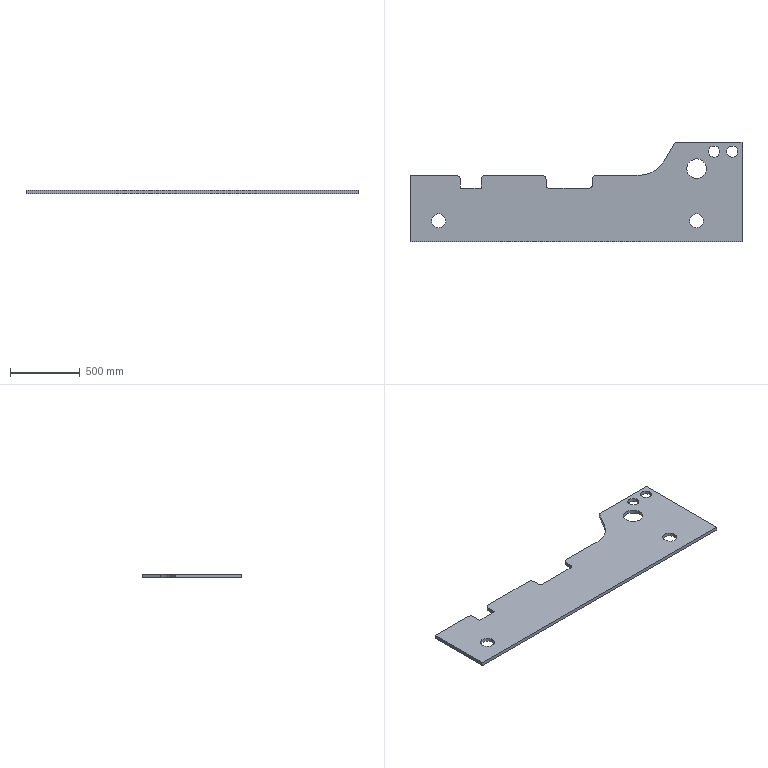Part | SolidWorks | features Extrusion 1 | 1 solid | 33 faces | box 2375 x 714.5 x 25 mm | volume 29470631 mm3 | cylinder 17 | plane 16 | commonest cylinder face diameters 60 x4 80 x4 100 x4 40 x2 140 x2 418 x1
STEP:
#1=CARTESIAN_POINT('',(155.,151.5,25.));
#2=VERTEX_POINT('',#1);
#3=CARTESIAN_POINT('',(255.,151.5,25.));
#4=VERTEX_POINT('',#3);
#5=CARTESIAN_POINT('',(205.,151.5,25.));
#6=DIRECTION('',(0.,0.,1.));
#7=DIRECTION('',(1.,0.,0.));
#8=AXIS2_PLACEMENT_3D('',#5,#6,#7);
#9=CIRCLE('',#8,50.);
#10=EDGE_CURVE('',#2,#4,#9,.T.);
#11=ORIENTED_EDGE('',*,*,#10,.T.);
#12=CARTESIAN_POINT('',(255.,151.5,0.));
#13=VERTEX_POINT('',#12);
#14=CARTESIAN_POINT('',(255.,151.5,25.));
#15=DIRECTION('',(0.,0.,-1.));
#16=VECTOR('',#15,1000.);
#17=LINE('',#14,#16);
#18=EDGE_CURVE('',#4,#13,#17,.T.);
#19=ORIENTED_EDGE('',*,*,#18,.T.);
#20=CARTESIAN_POINT('',(155.,151.5,0.));
#21=VERTEX_POINT('',#20);
#22=CARTESIAN_POINT('',(205.,151.5,0.));
#23=DIRECTION('',(0.,0.,1.));
#24=DIRECTION('',(1.,0.,0.));
#25=AXIS2_PLACEMENT_3D('',#22,#23,#24);
#26=CIRCLE('',#25,50.);
#27=EDGE_CURVE('',#21,#13,#26,.T.);
#28=ORIENTED_EDGE('',*,*,#27,.F.);
#29=CARTESIAN_POINT('',(155.,151.5,25.));
#30=DIRECTION('',(0.,0.,-1.));
#31=VECTOR('',#30,1000.);
#32=LINE('',#29,#31);
#33=EDGE_CURVE('',#2,#21,#32,.T.);
#34=ORIENTED_EDGE('',*,*,#33,.F.);
#35=EDGE_LOOP('',(#11,#19,#28,#34));
#36=FACE_OUTER_BOUND('',#35,.T.);
#37=CARTESIAN_POINT('',(205.,151.5,25.));
#38=DIRECTION('',(0.,0.,-1.));
#39=DIRECTION('',(-1.,0.,0.));
#40=AXIS2_PLACEMENT_3D('',#37,#38,#39);
#41=CYLINDRICAL_SURFACE('',#40,50.);
#42=ADVANCED_FACE('',(#36),#41,.F.);
#43=CARTESIAN_POINT('',(2135.,646.5,25.));
#44=VERTEX_POINT('',#43);
#45=CARTESIAN_POINT('',(2215.,646.5,25.));
#46=VERTEX_POINT('',#45);
#47=CARTESIAN_POINT('',(2175.,646.5,25.));
#48=DIRECTION('',(0.,0.,1.));
#49=DIRECTION('',(1.,0.,0.));
#50=AXIS2_PLACEMENT_3D('',#47,#48,#49);
#51=CIRCLE('',#50,40.);
#52=EDGE_CURVE('',#44,#46,#51,.T.);
#53=ORIENTED_EDGE('',*,*,#52,.T.);
#54=CARTESIAN_POINT('',(2215.,646.5,0.));
#55=VERTEX_POINT('',#54);
#56=CARTESIAN_POINT('',(2215.,646.5,25.));
#57=DIRECTION('',(0.,0.,-1.));
#58=VECTOR('',#57,1000.);
#59=LINE('',#56,#58);
#60=EDGE_CURVE('',#46,#55,#59,.T.);
#61=ORIENTED_EDGE('',*,*,#60,.T.);
#62=CARTESIAN_POINT('',(2135.,646.5,0.));
#63=VERTEX_POINT('',#62);
#64=CARTESIAN_POINT('',(2175.,646.5,0.));
#65=DIRECTION('',(0.,0.,1.));
#66=DIRECTION('',(1.,0.,0.));
#67=AXIS2_PLACEMENT_3D('',#64,#65,#66);
#68=CIRCLE('',#67,40.);
#69=EDGE_CURVE('',#63,#55,#68,.T.);
#70=ORIENTED_EDGE('',*,*,#69,.F.);
#71=CARTESIAN_POINT('',(2135.,646.5,25.));
#72=DIRECTION('',(0.,0.,-1.));
#73=VECTOR('',#72,1000.);
#74=LINE('',#71,#73);
#75=EDGE_CURVE('',#44,#63,#74,.T.);
#76=ORIENTED_EDGE('',*,*,#75,.F.);
#77=EDGE_LOOP('',(#53,#61,#70,#76));
#78=FACE_OUTER_BOUND('',#77,.T.);
#79=CARTESIAN_POINT('',(2175.,646.5,25.));
#80=DIRECTION('',(0.,0.,-1.));
#81=DIRECTION('',(-1.,0.,0.));
#82=AXIS2_PLACEMENT_3D('',#79,#80,#81);
#83=CYLINDRICAL_SURFACE('',#82,40.);
#84=ADVANCED_FACE('',(#78),#83,.F.);
#85=CARTESIAN_POINT('',(2265.,646.5,25.));
#86=VERTEX_POINT('',#85);
#87=CARTESIAN_POINT('',(2345.,646.5,25.));
#88=VERTEX_POINT('',#87);
#89=CARTESIAN_POINT('',(2305.,646.5,25.));
#90=DIRECTION('',(0.,0.,1.));
#91=DIRECTION('',(1.,0.,0.));
#92=AXIS2_PLACEMENT_3D('',#89,#90,#91);
#93=CIRCLE('',#92,40.);
#94=EDGE_CURVE('',#86,#88,#93,.T.);
#95=ORIENTED_EDGE('',*,*,#94,.T.);
#96=CARTESIAN_POINT('',(2345.,646.5,0.));
#97=VERTEX_POINT('',#96);
#98=CARTESIAN_POINT('',(2345.,646.5,25.));
#99=DIRECTION('',(0.,0.,-1.));
#100=VECTOR('',#99,1000.);
#101=LINE('',#98,#100);
#102=EDGE_CURVE('',#88,#97,#101,.T.);
#103=ORIENTED_EDGE('',*,*,#102,.T.);
#104=CARTESIAN_POINT('',(2265.,646.5,0.));
#105=VERTEX_POINT('',#104);
#106=CARTESIAN_POINT('',(2305.,646.5,0.));
#107=DIRECTION('',(0.,0.,1.));
#108=DIRECTION('',(1.,0.,0.));
#109=AXIS2_PLACEMENT_3D('',#106,#107,#108);
#110=CIRCLE('',#109,40.);
#111=EDGE_CURVE('',#105,#97,#110,.T.);
#112=ORIENTED_EDGE('',*,*,#111,.F.);
#113=CARTESIAN_POINT('',(2265.,646.5,25.));
#114=DIRECTION('',(0.,0.,-1.));
#115=VECTOR('',#114,1000.);
#116=LINE('',#113,#115);
#117=EDGE_CURVE('',#86,#105,#116,.T.);
#118=ORIENTED_EDGE('',*,*,#117,.F.);
#119=EDGE_LOOP('',(#95,#103,#112,#118));
#120=FACE_OUTER_BOUND('',#119,.T.);
#121=CARTESIAN_POINT('',(2305.,646.5,25.));
#122=DIRECTION('',(0.,0.,-1.));
#123=DIRECTION('',(-1.,0.,0.));
#124=AXIS2_PLACEMENT_3D('',#121,#122,#123);
#125=CYLINDRICAL_SURFACE('',#124,40.);
#126=ADVANCED_FACE('',(#120),#125,.F.);
#127=CARTESIAN_POINT('',(1980.,524.5,25.));
#128=VERTEX_POINT('',#127);
#129=CARTESIAN_POINT('',(2120.,524.5,25.));
#130=VERTEX_POINT('',#129);
#131=CARTESIAN_POINT('',(2050.,524.5,25.));
#132=DIRECTION('',(0.,0.,1.));
#133=DIRECTION('',(1.,0.,0.));
#134=AXIS2_PLACEMENT_3D('',#131,#132,#133);
#135=CIRCLE('',#134,70.);
#136=EDGE_CURVE('',#128,#130,#135,.T.);
#137=ORIENTED_EDGE('',*,*,#136,.T.);
#138=CARTESIAN_POINT('',(2120.,524.5,0.));
#139=VERTEX_POINT('',#138);
#140=CARTESIAN_POINT('',(2120.,524.5,25.));
#141=DIRECTION('',(0.,0.,-1.));
#142=VECTOR('',#141,1000.);
#143=LINE('',#140,#142);
#144=EDGE_CURVE('',#130,#139,#143,.T.);
#145=ORIENTED_EDGE('',*,*,#144,.T.);
#146=CARTESIAN_POINT('',(1980.,524.5,0.));
#147=VERTEX_POINT('',#146);
#148=CARTESIAN_POINT('',(2050.,524.5,0.));
#149=DIRECTION('',(0.,0.,1.));
#150=DIRECTION('',(1.,0.,0.));
#151=AXIS2_PLACEMENT_3D('',#148,#149,#150);
#152=CIRCLE('',#151,70.);
#153=EDGE_CURVE('',#147,#139,#152,.T.);
#154=ORIENTED_EDGE('',*,*,#153,.F.);
#155=CARTESIAN_POINT('',(1980.,524.5,25.));
#156=DIRECTION('',(0.,0.,-1.));
#157=VECTOR('',#156,1000.);
#158=LINE('',#155,#157);
#159=EDGE_CURVE('',#128,#147,#158,.T.);
#160=ORIENTED_EDGE('',*,*,#159,.F.);
#161=EDGE_LOOP('',(#137,#145,#154,#160));
#162=FACE_OUTER_BOUND('',#161,.T.);
#163=CARTESIAN_POINT('',(2050.,524.5,25.));
#164=DIRECTION('',(0.,0.,-1.));
#165=DIRECTION('',(-1.,0.,0.));
#166=AXIS2_PLACEMENT_3D('',#163,#164,#165);
#167=CYLINDRICAL_SURFACE('',#166,70.);
#168=ADVANCED_FACE('',(#162),#167,.F.);
#169=CARTESIAN_POINT('',(2000.,151.5,25.));
#170=VERTEX_POINT('',#169);
#171=CARTESIAN_POINT('',(2100.,151.5,25.));
#172=VERTEX_POINT('',#171);
#173=CARTESIAN_POINT('',(2050.,151.5,25.));
#174=DIRECTION('',(0.,0.,1.));
#175=DIRECTION('',(1.,0.,0.));
#176=AXIS2_PLACEMENT_3D('',#173,#174,#175);
#177=CIRCLE('',#176,50.);
#178=EDGE_CURVE('',#170,#172,#177,.T.);
#179=ORIENTED_EDGE('',*,*,#178,.T.);
#180=CARTESIAN_POINT('',(2100.,151.5,0.));
#181=VERTEX_POINT('',#180);
#182=CARTESIAN_POINT('',(2100.,151.5,25.));
#183=DIRECTION('',(0.,0.,-1.));
#184=VECTOR('',#183,1000.);
#185=LINE('',#182,#184);
#186=EDGE_CURVE('',#172,#181,#185,.T.);
#187=ORIENTED_EDGE('',*,*,#186,.T.);
#188=CARTESIAN_POINT('',(2000.,151.5,0.));
#189=VERTEX_POINT('',#188);
#190=CARTESIAN_POINT('',(2050.,151.5,0.));
#191=DIRECTION('',(0.,0.,1.));
#192=DIRECTION('',(1.,0.,0.));
#193=AXIS2_PLACEMENT_3D('',#190,#191,#192);
#194=CIRCLE('',#193,50.);
#195=EDGE_CURVE('',#189,#181,#194,.T.);
#196=ORIENTED_EDGE('',*,*,#195,.F.);
#197=CARTESIAN_POINT('',(2000.,151.5,25.));
#198=DIRECTION('',(0.,0.,-1.));
#199=VECTOR('',#198,1000.);
#200=LINE('',#197,#199);
#201=EDGE_CURVE('',#170,#189,#200,.T.);
#202=ORIENTED_EDGE('',*,*,#201,.F.);
#203=EDGE_LOOP('',(#179,#187,#196,#202));
#204=FACE_OUTER_BOUND('',#203,.T.);
#205=CARTESIAN_POINT('',(2050.,151.5,25.));
#206=DIRECTION('',(0.,0.,-1.));
#207=DIRECTION('',(-1.,0.,0.));
#208=AXIS2_PLACEMENT_3D('',#205,#206,#207);
#209=CYLINDRICAL_SURFACE('',#208,50.);
#210=ADVANCED_FACE('',(#204),#209,.F.);
#211=CARTESIAN_POINT('',(330.,477.,0.));
#212=VERTEX_POINT('',#211);
#213=CARTESIAN_POINT('',(360.,447.,0.));
#214=VERTEX_POINT('',#213);
#215=CARTESIAN_POINT('',(330.,447.,0.));
#216=DIRECTION('',(0.,0.,-1.));
#217=DIRECTION('',(1.,0.,0.));
#218=AXIS2_PLACEMENT_3D('',#215,#216,#217);
#219=CIRCLE('',#218,30.);
#220=EDGE_CURVE('',#212,#214,#219,.T.);
#221=ORIENTED_EDGE('',*,*,#220,.F.);
#222=CARTESIAN_POINT('',(330.,477.,25.));
#223=VERTEX_POINT('',#222);
#224=CARTESIAN_POINT('',(330.,477.,25.));
#225=DIRECTION('',(0.,0.,-1.));
#226=VECTOR('',#225,1000.);
#227=LINE('',#224,#226);
#228=EDGE_CURVE('',#223,#212,#227,.T.);
#229=ORIENTED_EDGE('',*,*,#228,.F.);
#230=CARTESIAN_POINT('',(360.,447.,25.));
#231=VERTEX_POINT('',#230);
#232=CARTESIAN_POINT('',(330.,447.,25.));
#233=DIRECTION('',(0.,0.,-1.));
#234=DIRECTION('',(1.,0.,0.));
#235=AXIS2_PLACEMENT_3D('',#232,#233,#234);
#236=CIRCLE('',#235,30.);
#237=EDGE_CURVE('',#223,#231,#236,.T.);
#238=ORIENTED_EDGE('',*,*,#237,.T.);
#239=CARTESIAN_POINT('',(360.,447.,25.));
#240=DIRECTION('',(0.,0.,-1.));
#241=VECTOR('',#240,1000.);
#242=LINE('',#239,#241);
#243=EDGE_CURVE('',#231,#214,#242,.T.);
#244=ORIENTED_EDGE('',*,*,#243,.T.);
#245=EDGE_LOOP('',(#221,#229,#238,#244));
#246=FACE_OUTER_BOUND('',#245,.T.);
#247=CARTESIAN_POINT('',(330.,447.,25.));
#248=DIRECTION('',(0.,0.,-1.));
#249=DIRECTION('',(-1.,0.,0.));
#250=AXIS2_PLACEMENT_3D('',#247,#248,#249);
#251=CYLINDRICAL_SURFACE('',#250,30.);
#252=ADVANCED_FACE('',(#246),#251,.T.);
#253=CARTESIAN_POINT('',(0.,477.,0.));
#254=VERTEX_POINT('',#253);
#255=CARTESIAN_POINT('',(1187.432,477.,0.));
#256=DIRECTION('',(1.,0.,0.));
#257=VECTOR('',#256,1000.);
#258=LINE('',#255,#257);
#259=EDGE_CURVE('',#254,#212,#258,.T.);
#260=ORIENTED_EDGE('',*,*,#259,.F.);
#261=CARTESIAN_POINT('',(0.,477.,25.));
#262=VERTEX_POINT('',#261);
#263=CARTESIAN_POINT('',(0.,477.,25.));
#264=DIRECTION('',(0.,0.,-1.));
#265=VECTOR('',#264,1000.);
#266=LINE('',#263,#265);
#267=EDGE_CURVE('',#262,#254,#266,.T.);
#268=ORIENTED_EDGE('',*,*,#267,.F.);
#269=CARTESIAN_POINT('',(1187.432,477.,25.));
#270=DIRECTION('',(1.,0.,0.));
#271=VECTOR('',#270,1000.);
#272=LINE('',#269,#271);
#273=EDGE_CURVE('',#262,#223,#272,.T.);
#274=ORIENTED_EDGE('',*,*,#273,.T.);
#275=ORIENTED_EDGE('',*,*,#228,.T.);
#276=EDGE_LOOP('',(#260,#268,#274,#275));
#277=FACE_OUTER_BOUND('',#276,.T.);
#278=CARTESIAN_POINT('',(1187.432,477.,25.));
#279=DIRECTION('',(0.,1.,0.));
#280=DIRECTION('',(0.,0.,1.));
#281=AXIS2_PLACEMENT_3D('',#278,#279,#280);
#282=PLANE('',#281);
#283=ADVANCED_FACE('',(#277),#282,.T.);
#284=CARTESIAN_POINT('',(0.,0.,0.));
#285=VERTEX_POINT('',#284);
#286=CARTESIAN_POINT('',(0.,-1572.124,0.));
#287=DIRECTION('',(0.,1.,0.));
#288=VECTOR('',#287,1000.);
#289=LINE('',#286,#288);
#290=EDGE_CURVE('',#285,#254,#289,.T.);
#291=ORIENTED_EDGE('',*,*,#290,.F.);
#292=CARTESIAN_POINT('',(0.,0.,25.));
#293=VERTEX_POINT('',#292);
#294=CARTESIAN_POINT('',(0.,0.,25.));
#295=DIRECTION('',(0.,0.,-1.));
#296=VECTOR('',#295,1000.);
#297=LINE('',#294,#296);
#298=EDGE_CURVE('',#293,#285,#297,.T.);
#299=ORIENTED_EDGE('',*,*,#298,.F.);
#300=CARTESIAN_POINT('',(0.,-1572.124,25.));
#301=DIRECTION('',(0.,1.,0.));
#302=VECTOR('',#301,1000.);
#303=LINE('',#300,#302);
#304=EDGE_CURVE('',#293,#262,#303,.T.);
#305=ORIENTED_EDGE('',*,*,#304,.T.);
#306=ORIENTED_EDGE('',*,*,#267,.T.);
#307=EDGE_LOOP('',(#291,#299,#305,#306));
#308=FACE_OUTER_BOUND('',#307,.T.);
#309=CARTESIAN_POINT('',(0.,-1572.124,25.));
#310=DIRECTION('',(-1.,0.,0.));
#311=DIRECTION('',(0.,0.,1.));
#312=AXIS2_PLACEMENT_3D('',#309,#310,#311);
#313=PLANE('',#312);
#314=ADVANCED_FACE('',(#308),#313,.T.);
#315=CARTESIAN_POINT('',(2375.,0.,0.));
#316=VERTEX_POINT('',#315);
#317=CARTESIAN_POINT('',(1187.432,0.,0.));
#318=DIRECTION('',(-1.,0.,0.));
#319=VECTOR('',#318,1000.);
#320=LINE('',#317,#319);
#321=EDGE_CURVE('',#316,#285,#320,.T.);
#322=ORIENTED_EDGE('',*,*,#321,.F.);
#323=CARTESIAN_POINT('',(2375.,0.,25.));
#324=VERTEX_POINT('',#323);
#325=CARTESIAN_POINT('',(2375.,0.,25.));
#326=DIRECTION('',(0.,0.,-1.));
#327=VECTOR('',#326,1000.);
#328=LINE('',#325,#327);
#329=EDGE_CURVE('',#324,#316,#328,.T.);
#330=ORIENTED_EDGE('',*,*,#329,.F.);
#331=CARTESIAN_POINT('',(1187.432,0.,25.));
#332=DIRECTION('',(-1.,0.,0.));
#333=VECTOR('',#332,1000.);
#334=LINE('',#331,#333);
#335=EDGE_CURVE('',#324,#293,#334,.T.);
#336=ORIENTED_EDGE('',*,*,#335,.T.);
#337=ORIENTED_EDGE('',*,*,#298,.T.);
#338=EDGE_LOOP('',(#322,#330,#336,#337));
#339=FACE_OUTER_BOUND('',#338,.T.);
#340=CARTESIAN_POINT('',(1187.432,0.,25.));
#341=DIRECTION('',(0.,-1.,0.));
#342=DIRECTION('',(1.,0.,0.));
#343=AXIS2_PLACEMENT_3D('',#340,#341,#342);
#344=PLANE('',#343);
#345=ADVANCED_FACE('',(#339),#344,.T.);
#346=CARTESIAN_POINT('',(2375.,714.5,0.));
#347=VERTEX_POINT('',#346);
#348=CARTESIAN_POINT('',(2375.,-1572.124,0.));
#349=DIRECTION('',(0.,-1.,0.));
#350=VECTOR('',#349,1000.);
#351=LINE('',#348,#350);
#352=EDGE_CURVE('',#347,#316,#351,.T.);
#353=ORIENTED_EDGE('',*,*,#352,.F.);
#354=CARTESIAN_POINT('',(2375.,714.5,25.));
#355=VERTEX_POINT('',#354);
#356=CARTESIAN_POINT('',(2375.,714.5,25.));
#357=DIRECTION('',(0.,0.,-1.));
#358=VECTOR('',#357,1000.);
#359=LINE('',#356,#358);
#360=EDGE_CURVE('',#355,#347,#359,.T.);
#361=ORIENTED_EDGE('',*,*,#360,.F.);
#362=CARTESIAN_POINT('',(2375.,-1572.124,25.));
#363=DIRECTION('',(0.,-1.,0.));
#364=VECTOR('',#363,1000.);
#365=LINE('',#362,#364);
#366=EDGE_CURVE('',#355,#324,#365,.T.);
#367=ORIENTED_EDGE('',*,*,#366,.T.);
#368=ORIENTED_EDGE('',*,*,#329,.T.);
#369=EDGE_LOOP('',(#353,#361,#367,#368));
#370=FACE_OUTER_BOUND('',#369,.T.);
#371=CARTESIAN_POINT('',(2375.,-1572.124,25.));
#372=DIRECTION('',(1.,0.,0.));
#373=DIRECTION('',(0.,0.,-1.));
#374=AXIS2_PLACEMENT_3D('',#371,#372,#373);
#375=PLANE('',#374);
#376=ADVANCED_FACE('',(#370),#375,.T.);
#377=CARTESIAN_POINT('',(1896.2,714.5,0.));
#378=VERTEX_POINT('',#377);
#379=CARTESIAN_POINT('',(1187.432,714.5,0.));
#380=DIRECTION('',(1.,0.,0.));
#381=VECTOR('',#380,1000.);
#382=LINE('',#379,#381);
#383=EDGE_CURVE('',#378,#347,#382,.T.);
#384=ORIENTED_EDGE('',*,*,#383,.F.);
#385=CARTESIAN_POINT('',(1896.2,714.5,25.));
#386=VERTEX_POINT('',#385);
#387=CARTESIAN_POINT('',(1896.2,714.5,25.));
#388=DIRECTION('',(0.,0.,-1.));
#389=VECTOR('',#388,1000.);
#390=LINE('',#387,#389);
#391=EDGE_CURVE('',#386,#378,#390,.T.);
#392=ORIENTED_EDGE('',*,*,#391,.F.);
#393=CARTESIAN_POINT('',(1187.432,714.5,25.));
#394=DIRECTION('',(1.,0.,0.));
#395=VECTOR('',#394,1000.);
#396=LINE('',#393,#395);
#397=EDGE_CURVE('',#386,#355,#396,.T.);
#398=ORIENTED_EDGE('',*,*,#397,.T.);
#399=ORIENTED_EDGE('',*,*,#360,.T.);
#400=EDGE_LOOP('',(#384,#392,#398,#399));
#401=FACE_OUTER_BOUND('',#400,.T.);
#402=CARTESIAN_POINT('',(1187.432,714.5,25.));
#403=DIRECTION('',(0.,1.,0.));
#404=DIRECTION('',(0.,0.,1.));
#405=AXIS2_PLACEMENT_3D('',#402,#403,#404);
#406=PLANE('',#405);
#407=ADVANCED_FACE('',(#401),#406,.T.);
#408=CARTESIAN_POINT('',(1819.412,581.5,0.));
#409=VERTEX_POINT('',#408);
#410=CARTESIAN_POINT('',(728.871,-1307.374,0.));
#411=DIRECTION('',(-0.5,-0.866,0.));
#412=VECTOR('',#411,1000.);
#413=LINE('',#410,#412);
#414=EDGE_CURVE('',#378,#409,#413,.T.);
#415=ORIENTED_EDGE('',*,*,#414,.T.);
#416=CARTESIAN_POINT('',(1819.412,581.5,25.));
#417=VERTEX_POINT('',#416);
#418=CARTESIAN_POINT('',(1819.412,581.5,25.));
#419=DIRECTION('',(0.,0.,-1.));
#420=VECTOR('',#419,1000.);
#421=LINE('',#418,#420);
#422=EDGE_CURVE('',#417,#409,#421,.T.);
#423=ORIENTED_EDGE('',*,*,#422,.F.);
#424=CARTESIAN_POINT('',(728.871,-1307.374,25.));
#425=DIRECTION('',(-0.5,-0.866,0.));
#426=VECTOR('',#425,1000.);
#427=LINE('',#424,#426);
#428=EDGE_CURVE('',#386,#417,#427,.T.);
#429=ORIENTED_EDGE('',*,*,#428,.F.);
#430=ORIENTED_EDGE('',*,*,#391,.T.);
#431=EDGE_LOOP('',(#415,#423,#429,#430));
#432=FACE_OUTER_BOUND('',#431,.T.);
#433=CARTESIAN_POINT('',(728.871,-1307.374,25.));
#434=DIRECTION('',(0.866,-0.5,0.));
#435=DIRECTION('',(0.5,0.866,0.));
#436=AXIS2_PLACEMENT_3D('',#433,#434,#435);
#437=PLANE('',#436);
#438=ADVANCED_FACE('',(#432),#437,.F.);
#439=CARTESIAN_POINT('',(1638.413,477.,0.));
#440=VERTEX_POINT('',#439);
#441=CARTESIAN_POINT('',(1638.413,686.,0.));
#442=DIRECTION('',(0.,0.,-1.));
#443=DIRECTION('',(1.,0.,0.));
#444=AXIS2_PLACEMENT_3D('',#441,#442,#443);
#445=CIRCLE('',#444,209.);
#446=EDGE_CURVE('',#409,#440,#445,.T.);
#447=ORIENTED_EDGE('',*,*,#446,.T.);
#448=CARTESIAN_POINT('',(1638.413,477.,25.));
#449=VERTEX_POINT('',#448);
#450=CARTESIAN_POINT('',(1638.413,477.,25.));
#451=DIRECTION('',(0.,0.,-1.));
#452=VECTOR('',#451,1000.);
#453=LINE('',#450,#452);
#454=EDGE_CURVE('',#449,#440,#453,.T.);
#455=ORIENTED_EDGE('',*,*,#454,.F.);
#456=CARTESIAN_POINT('',(1638.413,686.,25.));
#457=DIRECTION('',(0.,0.,-1.));
#458=DIRECTION('',(1.,0.,0.));
#459=AXIS2_PLACEMENT_3D('',#456,#457,#458);
#460=CIRCLE('',#459,209.);
#461=EDGE_CURVE('',#417,#449,#460,.T.);
#462=ORIENTED_EDGE('',*,*,#461,.F.);
#463=ORIENTED_EDGE('',*,*,#422,.T.);
#464=EDGE_LOOP('',(#447,#455,#462,#463));
#465=FACE_OUTER_BOUND('',#464,.T.);
#466=CARTESIAN_POINT('',(1638.413,686.,25.));
#467=DIRECTION('',(0.,0.,-1.));
#468=DIRECTION('',(-1.,0.,0.));
#469=AXIS2_PLACEMENT_3D('',#466,#467,#468);
#470=CYLINDRICAL_SURFACE('',#469,209.);
#471=ADVANCED_FACE('',(#465),#470,.F.);
#472=CARTESIAN_POINT('',(1333.,477.,0.));
#473=VERTEX_POINT('',#472);
#474=CARTESIAN_POINT('',(1187.432,477.,0.));
#475=DIRECTION('',(1.,0.,0.));
#476=VECTOR('',#475,1000.);
#477=LINE('',#474,#476);
#478=EDGE_CURVE('',#473,#440,#477,.T.);
#479=ORIENTED_EDGE('',*,*,#478,.F.);
#480=CARTESIAN_POINT('',(1333.,477.,25.));
#481=VERTEX_POINT('',#480);
#482=CARTESIAN_POINT('',(1333.,477.,25.));
#483=DIRECTION('',(0.,0.,-1.));
#484=VECTOR('',#483,1000.);
#485=LINE('',#482,#484);
#486=EDGE_CURVE('',#481,#473,#485,.T.);
#487=ORIENTED_EDGE('',*,*,#486,.F.);
#488=CARTESIAN_POINT('',(1187.432,477.,25.));
#489=DIRECTION('',(1.,0.,0.));
#490=VECTOR('',#489,1000.);
#491=LINE('',#488,#490);
#492=EDGE_CURVE('',#481,#449,#491,.T.);
#493=ORIENTED_EDGE('',*,*,#492,.T.);
#494=ORIENTED_EDGE('',*,*,#454,.T.);
#495=EDGE_LOOP('',(#479,#487,#493,#494));
#496=FACE_OUTER_BOUND('',#495,.T.);
#497=CARTESIAN_POINT('',(1187.432,477.,25.));
#498=DIRECTION('',(0.,1.,0.));
#499=DIRECTION('',(-1.,0.,0.));
#500=AXIS2_PLACEMENT_3D('',#497,#498,#499);
#501=PLANE('',#500);
#502=ADVANCED_FACE('',(#496),#501,.T.);
#503=CARTESIAN_POINT('',(1303.,447.,0.));
#504=VERTEX_POINT('',#503);
#505=CARTESIAN_POINT('',(1333.,447.,0.));
#506=DIRECTION('',(0.,0.,-1.));
#507=DIRECTION('',(1.,0.,0.));
#508=AXIS2_PLACEMENT_3D('',#505,#506,#507);
#509=CIRCLE('',#508,30.);
#510=EDGE_CURVE('',#504,#473,#509,.T.);
#511=ORIENTED_EDGE('',*,*,#510,.F.);
#512=CARTESIAN_POINT('',(1303.,447.,25.));
#513=VERTEX_POINT('',#512);
#514=CARTESIAN_POINT('',(1303.,447.,25.));
#515=DIRECTION('',(0.,0.,-1.));
#516=VECTOR('',#515,1000.);
#517=LINE('',#514,#516);
#518=EDGE_CURVE('',#513,#504,#517,.T.);
#519=ORIENTED_EDGE('',*,*,#518,.F.);
#520=CARTESIAN_POINT('',(1333.,447.,25.));
#521=DIRECTION('',(0.,0.,-1.));
#522=DIRECTION('',(1.,0.,0.));
#523=AXIS2_PLACEMENT_3D('',#520,#521,#522);
#524=CIRCLE('',#523,30.);
#525=EDGE_CURVE('',#513,#481,#524,.T.);
#526=ORIENTED_EDGE('',*,*,#525,.T.);
#527=ORIENTED_EDGE('',*,*,#486,.T.);
#528=EDGE_LOOP('',(#511,#519,#526,#527));
#529=FACE_OUTER_BOUND('',#528,.T.);
#530=CARTESIAN_POINT('',(1333.,447.,25.));
#531=DIRECTION('',(0.,0.,-1.));
#532=DIRECTION('',(-1.,0.,0.));
#533=AXIS2_PLACEMENT_3D('',#530,#531,#532);
#534=CYLINDRICAL_SURFACE('',#533,30.);
#535=ADVANCED_FACE('',(#529),#534,.T.);
#536=CARTESIAN_POINT('',(1303.,404.,0.));
#537=VERTEX_POINT('',#536);
#538=CARTESIAN_POINT('',(1303.,-1572.124,0.));
#539=DIRECTION('',(0.,1.,0.));
#540=VECTOR('',#539,1000.);
#541=LINE('',#538,#540);
#542=EDGE_CURVE('',#537,#504,#541,.T.);
#543=ORIENTED_EDGE('',*,*,#542,.F.);
#544=CARTESIAN_POINT('',(1303.,404.,25.));
#545=VERTEX_POINT('',#544);
#546=CARTESIAN_POINT('',(1303.,404.,25.));
#547=DIRECTION('',(0.,0.,-1.));
#548=VECTOR('',#547,1000.);
#549=LINE('',#546,#548);
#550=EDGE_CURVE('',#545,#537,#549,.T.);
#551=ORIENTED_EDGE('',*,*,#550,.F.);
#552=CARTESIAN_POINT('',(1303.,-1572.124,25.));
#553=DIRECTION('',(0.,1.,0.));
#554=VECTOR('',#553,1000.);
#555=LINE('',#552,#554);
#556=EDGE_CURVE('',#545,#513,#555,.T.);
#557=ORIENTED_EDGE('',*,*,#556,.T.);
#558=ORIENTED_EDGE('',*,*,#518,.T.);
#559=EDGE_LOOP('',(#543,#551,#557,#558));
#560=FACE_OUTER_BOUND('',#559,.T.);
#561=CARTESIAN_POINT('',(1303.,-1572.124,25.));
#562=DIRECTION('',(-1.,0.,0.));
#563=DIRECTION('',(0.,0.,1.));
#564=AXIS2_PLACEMENT_3D('',#561,#562,#563);
#565=PLANE('',#564);
#566=ADVANCED_FACE('',(#560),#565,.T.);
#567=CARTESIAN_POINT('',(1283.,384.,0.));
#568=VERTEX_POINT('',#567);
#569=CARTESIAN_POINT('',(1283.,404.,0.));
#570=DIRECTION('',(0.,0.,-1.));
#571=DIRECTION('',(1.,0.,0.));
#572=AXIS2_PLACEMENT_3D('',#569,#570,#571);
#573=CIRCLE('',#572,20.);
#574=EDGE_CURVE('',#537,#568,#573,.T.);
#575=ORIENTED_EDGE('',*,*,#574,.T.);
#576=CARTESIAN_POINT('',(1283.,384.,25.));
#577=VERTEX_POINT('',#576);
#578=CARTESIAN_POINT('',(1283.,384.,25.));
#579=DIRECTION('',(0.,0.,-1.));
#580=VECTOR('',#579,1000.);
#581=LINE('',#578,#580);
#582=EDGE_CURVE('',#577,#568,#581,.T.);
#583=ORIENTED_EDGE('',*,*,#582,.F.);
#584=CARTESIAN_POINT('',(1283.,404.,25.));
#585=DIRECTION('',(0.,0.,-1.));
#586=DIRECTION('',(1.,0.,0.));
#587=AXIS2_PLACEMENT_3D('',#584,#585,#586);
#588=CIRCLE('',#587,20.);
#589=EDGE_CURVE('',#545,#577,#588,.T.);
#590=ORIENTED_EDGE('',*,*,#589,.F.);
#591=ORIENTED_EDGE('',*,*,#550,.T.);
#592=EDGE_LOOP('',(#575,#583,#590,#591));
#593=FACE_OUTER_BOUND('',#592,.T.);
#594=CARTESIAN_POINT('',(1283.,404.,25.));
#595=DIRECTION('',(0.,0.,-1.));
#596=DIRECTION('',(-1.,0.,0.));
#597=AXIS2_PLACEMENT_3D('',#594,#595,#596);
#598=CYLINDRICAL_SURFACE('',#597,20.);
#599=ADVANCED_FACE('',(#593),#598,.F.);
#600=CARTESIAN_POINT('',(993.,384.,0.));
#601=VERTEX_POINT('',#600);
#602=CARTESIAN_POINT('',(1187.432,384.,0.));
#603=DIRECTION('',(1.,0.,0.));
#604=VECTOR('',#603,1000.);
#605=LINE('',#602,#604);
#606=EDGE_CURVE('',#601,#568,#605,.T.);
#607=ORIENTED_EDGE('',*,*,#606,.F.);
#608=CARTESIAN_POINT('',(993.,384.,25.));
#609=VERTEX_POINT('',#608);
#610=CARTESIAN_POINT('',(993.,384.,25.));
#611=DIRECTION('',(0.,0.,-1.));
#612=VECTOR('',#611,1000.);
#613=LINE('',#610,#612);
#614=EDGE_CURVE('',#609,#601,#613,.T.);
#615=ORIENTED_EDGE('',*,*,#614,.F.);
#616=CARTESIAN_POINT('',(1187.432,384.,25.));
#617=DIRECTION('',(1.,0.,0.));
#618=VECTOR('',#617,1000.);
#619=LINE('',#616,#618);
#620=EDGE_CURVE('',#609,#577,#619,.T.);
#621=ORIENTED_EDGE('',*,*,#620,.T.);
#622=ORIENTED_EDGE('',*,*,#582,.T.);
#623=EDGE_LOOP('',(#607,#615,#621,#622));
#624=FACE_OUTER_BOUND('',#623,.T.);
#625=CARTESIAN_POINT('',(1187.432,384.,25.));
#626=DIRECTION('',(0.,1.,0.));
#627=DIRECTION('',(0.,0.,1.));
#628=AXIS2_PLACEMENT_3D('',#625,#626,#627);
#629=PLANE('',#628);
#630=ADVANCED_FACE('',(#624),#629,.T.);
#631=CARTESIAN_POINT('',(973.,404.,0.));
#632=VERTEX_POINT('',#631);
#633=CARTESIAN_POINT('',(993.,404.,0.));
#634=DIRECTION('',(0.,0.,1.));
#635=DIRECTION('',(1.,0.,0.));
#636=AXIS2_PLACEMENT_3D('',#633,#634,#635);
#637=CIRCLE('',#636,20.);
#638=EDGE_CURVE('',#632,#601,#637,.T.);
#639=ORIENTED_EDGE('',*,*,#638,.F.);
#640=CARTESIAN_POINT('',(973.,404.,25.));
#641=VERTEX_POINT('',#640);
#642=CARTESIAN_POINT('',(973.,404.,25.));
#643=DIRECTION('',(0.,0.,-1.));
#644=VECTOR('',#643,1000.);
#645=LINE('',#642,#644);
#646=EDGE_CURVE('',#641,#632,#645,.T.);
#647=ORIENTED_EDGE('',*,*,#646,.F.);
#648=CARTESIAN_POINT('',(993.,404.,25.));
#649=DIRECTION('',(0.,0.,1.));
#650=DIRECTION('',(1.,0.,0.));
#651=AXIS2_PLACEMENT_3D('',#648,#649,#650);
#652=CIRCLE('',#651,20.);
#653=EDGE_CURVE('',#641,#609,#652,.T.);
#654=ORIENTED_EDGE('',*,*,#653,.T.);
#655=ORIENTED_EDGE('',*,*,#614,.T.);
#656=EDGE_LOOP('',(#639,#647,#654,#655));
#657=FACE_OUTER_BOUND('',#656,.T.);
#658=CARTESIAN_POINT('',(993.,404.,25.));
#659=DIRECTION('',(0.,0.,-1.));
#660=DIRECTION('',(-1.,0.,0.));
#661=AXIS2_PLACEMENT_3D('',#658,#659,#660);
#662=CYLINDRICAL_SURFACE('',#661,20.);
#663=ADVANCED_FACE('',(#657),#662,.F.);
#664=CARTESIAN_POINT('',(973.,447.,0.));
#665=VERTEX_POINT('',#664);
#666=CARTESIAN_POINT('',(973.,-1572.124,0.));
#667=DIRECTION('',(0.,-1.,0.));
#668=VECTOR('',#667,1000.);
#669=LINE('',#666,#668);
#670=EDGE_CURVE('',#665,#632,#669,.T.);
#671=ORIENTED_EDGE('',*,*,#670,.F.);
#672=CARTESIAN_POINT('',(973.,447.,25.));
#673=VERTEX_POINT('',#672);
#674=CARTESIAN_POINT('',(973.,447.,25.));
#675=DIRECTION('',(0.,0.,-1.));
#676=VECTOR('',#675,1000.);
#677=LINE('',#674,#676);
#678=EDGE_CURVE('',#673,#665,#677,.T.);
#679=ORIENTED_EDGE('',*,*,#678,.F.);
#680=CARTESIAN_POINT('',(973.,-1572.124,25.));
#681=DIRECTION('',(0.,-1.,0.));
#682=VECTOR('',#681,1000.);
#683=LINE('',#680,#682);
#684=EDGE_CURVE('',#673,#641,#683,.T.);
#685=ORIENTED_EDGE('',*,*,#684,.T.);
#686=ORIENTED_EDGE('',*,*,#646,.T.);
#687=EDGE_LOOP('',(#671,#679,#685,#686));
#688=FACE_OUTER_BOUND('',#687,.T.);
#689=CARTESIAN_POINT('',(973.,-1572.124,25.));
#690=DIRECTION('',(1.,0.,0.));
#691=DIRECTION('',(0.,0.,-1.));
#692=AXIS2_PLACEMENT_3D('',#689,#690,#691);
#693=PLANE('',#692);
#694=ADVANCED_FACE('',(#688),#693,.T.);
#695=CARTESIAN_POINT('',(943.,477.,0.));
#696=VERTEX_POINT('',#695);
#697=CARTESIAN_POINT('',(943.,447.,0.));
#698=DIRECTION('',(0.,0.,1.));
#699=DIRECTION('',(1.,0.,0.));
#700=AXIS2_PLACEMENT_3D('',#697,#698,#699);
#701=CIRCLE('',#700,30.);
#702=EDGE_CURVE('',#665,#696,#701,.T.);
#703=ORIENTED_EDGE('',*,*,#702,.T.);
#704=CARTESIAN_POINT('',(943.,477.,25.));
#705=VERTEX_POINT('',#704);
#706=CARTESIAN_POINT('',(943.,477.,25.));
#707=DIRECTION('',(0.,0.,-1.));
#708=VECTOR('',#707,1000.);
#709=LINE('',#706,#708);
#710=EDGE_CURVE('',#705,#696,#709,.T.);
#711=ORIENTED_EDGE('',*,*,#710,.F.);
#712=CARTESIAN_POINT('',(943.,447.,25.));
#713=DIRECTION('',(0.,0.,1.));
#714=DIRECTION('',(1.,0.,0.));
#715=AXIS2_PLACEMENT_3D('',#712,#713,#714);
#716=CIRCLE('',#715,30.);
#717=EDGE_CURVE('',#673,#705,#716,.T.);
#718=ORIENTED_EDGE('',*,*,#717,.F.);
#719=ORIENTED_EDGE('',*,*,#678,.T.);
#720=EDGE_LOOP('',(#703,#711,#718,#719));
#721=FACE_OUTER_BOUND('',#720,.T.);
#722=CARTESIAN_POINT('',(943.,447.,25.));
#723=DIRECTION('',(0.,0.,-1.));
#724=DIRECTION('',(-1.,0.,0.));
#725=AXIS2_PLACEMENT_3D('',#722,#723,#724);
#726=CYLINDRICAL_SURFACE('',#725,30.);
#727=ADVANCED_FACE('',(#721),#726,.T.);
#728=CARTESIAN_POINT('',(540.,477.,0.));
#729=VERTEX_POINT('',#728);
#730=CARTESIAN_POINT('',(1187.432,477.,0.));
#731=DIRECTION('',(1.,0.,0.));
#732=VECTOR('',#731,1000.);
#733=LINE('',#730,#732);
#734=EDGE_CURVE('',#729,#696,#733,.T.);
#735=ORIENTED_EDGE('',*,*,#734,.F.);
#736=CARTESIAN_POINT('',(540.,477.,25.));
#737=VERTEX_POINT('',#736);
#738=CARTESIAN_POINT('',(540.,477.,25.));
#739=DIRECTION('',(0.,0.,-1.));
#740=VECTOR('',#739,1000.);
#741=LINE('',#738,#740);
#742=EDGE_CURVE('',#737,#729,#741,.T.);
#743=ORIENTED_EDGE('',*,*,#742,.F.);
#744=CARTESIAN_POINT('',(1187.432,477.,25.));
#745=DIRECTION('',(1.,0.,0.));
#746=VECTOR('',#745,1000.);
#747=LINE('',#744,#746);
#748=EDGE_CURVE('',#737,#705,#747,.T.);
#749=ORIENTED_EDGE('',*,*,#748,.T.);
#750=ORIENTED_EDGE('',*,*,#710,.T.);
#751=EDGE_LOOP('',(#735,#743,#749,#750));
#752=FACE_OUTER_BOUND('',#751,.T.);
#753=CARTESIAN_POINT('',(1187.432,477.,25.));
#754=DIRECTION('',(0.,1.,0.));
#755=DIRECTION('',(0.,0.,1.));
#756=AXIS2_PLACEMENT_3D('',#753,#754,#755);
#757=PLANE('',#756);
#758=ADVANCED_FACE('',(#752),#757,.T.);
#759=CARTESIAN_POINT('',(510.,447.,0.));
#760=VERTEX_POINT('',#759);
#761=CARTESIAN_POINT('',(540.,447.,0.));
#762=DIRECTION('',(0.,0.,1.));
#763=DIRECTION('',(1.,0.,0.));
#764=AXIS2_PLACEMENT_3D('',#761,#762,#763);
#765=CIRCLE('',#764,30.);
#766=EDGE_CURVE('',#729,#760,#765,.T.);
#767=ORIENTED_EDGE('',*,*,#766,.T.);
#768=CARTESIAN_POINT('',(510.,447.,25.));
#769=VERTEX_POINT('',#768);
#770=CARTESIAN_POINT('',(510.,447.,25.));
#771=DIRECTION('',(0.,0.,-1.));
#772=VECTOR('',#771,1000.);
#773=LINE('',#770,#772);
#774=EDGE_CURVE('',#769,#760,#773,.T.);
#775=ORIENTED_EDGE('',*,*,#774,.F.);
#776=CARTESIAN_POINT('',(540.,447.,25.));
#777=DIRECTION('',(0.,0.,1.));
#778=DIRECTION('',(1.,0.,0.));
#779=AXIS2_PLACEMENT_3D('',#776,#777,#778);
#780=CIRCLE('',#779,30.);
#781=EDGE_CURVE('',#737,#769,#780,.T.);
#782=ORIENTED_EDGE('',*,*,#781,.F.);
#783=ORIENTED_EDGE('',*,*,#742,.T.);
#784=EDGE_LOOP('',(#767,#775,#782,#783));
#785=FACE_OUTER_BOUND('',#784,.T.);
#786=CARTESIAN_POINT('',(540.,447.,25.));
#787=DIRECTION('',(0.,0.,-1.));
#788=DIRECTION('',(-1.,0.,0.));
#789=AXIS2_PLACEMENT_3D('',#786,#787,#788);
#790=CYLINDRICAL_SURFACE('',#789,30.);
#791=ADVANCED_FACE('',(#785),#790,.T.);
#792=CARTESIAN_POINT('',(510.,384.,0.));
#793=VERTEX_POINT('',#792);
#794=CARTESIAN_POINT('',(510.,-1572.124,0.));
#795=DIRECTION('',(0.,1.,0.));
#796=VECTOR('',#795,1000.);
#797=LINE('',#794,#796);
#798=EDGE_CURVE('',#793,#760,#797,.T.);
#799=ORIENTED_EDGE('',*,*,#798,.F.);
#800=CARTESIAN_POINT('',(510.,384.,25.));
#801=VERTEX_POINT('',#800);
#802=CARTESIAN_POINT('',(510.,384.,25.));
#803=DIRECTION('',(0.,0.,-1.));
#804=VECTOR('',#803,1000.);
#805=LINE('',#802,#804);
#806=EDGE_CURVE('',#801,#793,#805,.T.);
#807=ORIENTED_EDGE('',*,*,#806,.F.);
#808=CARTESIAN_POINT('',(510.,-1572.124,25.));
#809=DIRECTION('',(0.,1.,0.));
#810=VECTOR('',#809,1000.);
#811=LINE('',#808,#810);
#812=EDGE_CURVE('',#801,#769,#811,.T.);
#813=ORIENTED_EDGE('',*,*,#812,.T.);
#814=ORIENTED_EDGE('',*,*,#774,.T.);
#815=EDGE_LOOP('',(#799,#807,#813,#814));
#816=FACE_OUTER_BOUND('',#815,.T.);
#817=CARTESIAN_POINT('',(510.,-1572.124,25.));
#818=DIRECTION('',(-1.,0.,0.));
#819=DIRECTION('',(0.,-1.,0.));
#820=AXIS2_PLACEMENT_3D('',#817,#818,#819);
#821=PLANE('',#820);
#822=ADVANCED_FACE('',(#816),#821,.T.);
#823=CARTESIAN_POINT('',(360.,384.,0.));
#824=VERTEX_POINT('',#823);
#825=CARTESIAN_POINT('',(1187.432,384.,0.));
#826=DIRECTION('',(-1.,0.,0.));
#827=VECTOR('',#826,1000.);
#828=LINE('',#825,#827);
#829=EDGE_CURVE('',#793,#824,#828,.T.);
#830=ORIENTED_EDGE('',*,*,#829,.T.);
#831=CARTESIAN_POINT('',(360.,384.,25.));
#832=VERTEX_POINT('',#831);
#833=CARTESIAN_POINT('',(360.,384.,25.));
#834=DIRECTION('',(0.,0.,-1.));
#835=VECTOR('',#834,1000.);
#836=LINE('',#833,#835);
#837=EDGE_CURVE('',#832,#824,#836,.T.);
#838=ORIENTED_EDGE('',*,*,#837,.F.);
#839=CARTESIAN_POINT('',(1187.432,384.,25.));
#840=DIRECTION('',(-1.,0.,0.));
#841=VECTOR('',#840,1000.);
#842=LINE('',#839,#841);
#843=EDGE_CURVE('',#801,#832,#842,.T.);
#844=ORIENTED_EDGE('',*,*,#843,.F.);
#845=ORIENTED_EDGE('',*,*,#806,.T.);
#846=EDGE_LOOP('',(#830,#838,#844,#845));
#847=FACE_OUTER_BOUND('',#846,.T.);
#848=CARTESIAN_POINT('',(1187.432,384.,25.));
#849=DIRECTION('',(0.,-1.,0.));
#850=DIRECTION('',(1.,0.,0.));
#851=AXIS2_PLACEMENT_3D('',#848,#849,#850);
#852=PLANE('',#851);
#853=ADVANCED_FACE('',(#847),#852,.F.);
#854=ORIENTED_EDGE('',*,*,#186,.F.);
#855=CARTESIAN_POINT('',(2050.,151.5,25.));
#856=DIRECTION('',(0.,0.,1.));
#857=DIRECTION('',(1.,0.,0.));
#858=AXIS2_PLACEMENT_3D('',#855,#856,#857);
#859=CIRCLE('',#858,50.);
#860=EDGE_CURVE('',#172,#170,#859,.T.);
#861=ORIENTED_EDGE('',*,*,#860,.T.);
#862=ORIENTED_EDGE('',*,*,#201,.T.);
#863=CARTESIAN_POINT('',(2050.,151.5,0.));
#864=DIRECTION('',(0.,0.,1.));
#865=DIRECTION('',(1.,0.,0.));
#866=AXIS2_PLACEMENT_3D('',#863,#864,#865);
#867=CIRCLE('',#866,50.);
#868=EDGE_CURVE('',#181,#189,#867,.T.);
#869=ORIENTED_EDGE('',*,*,#868,.F.);
#870=EDGE_LOOP('',(#854,#861,#862,#869));
#871=FACE_OUTER_BOUND('',#870,.T.);
#872=CARTESIAN_POINT('',(2050.,151.5,25.));
#873=DIRECTION('',(0.,0.,-1.));
#874=DIRECTION('',(-1.,0.,0.));
#875=AXIS2_PLACEMENT_3D('',#872,#873,#874);
#876=CYLINDRICAL_SURFACE('',#875,50.);
#877=ADVANCED_FACE('',(#871),#876,.F.);
#878=ORIENTED_EDGE('',*,*,#144,.F.);
#879=CARTESIAN_POINT('',(2050.,524.5,25.));
#880=DIRECTION('',(0.,0.,1.));
#881=DIRECTION('',(1.,0.,0.));
#882=AXIS2_PLACEMENT_3D('',#879,#880,#881);
#883=CIRCLE('',#882,70.);
#884=EDGE_CURVE('',#130,#128,#883,.T.);
#885=ORIENTED_EDGE('',*,*,#884,.T.);
#886=ORIENTED_EDGE('',*,*,#159,.T.);
#887=CARTESIAN_POINT('',(2050.,524.5,0.));
#888=DIRECTION('',(0.,0.,1.));
#889=DIRECTION('',(1.,0.,0.));
#890=AXIS2_PLACEMENT_3D('',#887,#888,#889);
#891=CIRCLE('',#890,70.);
#892=EDGE_CURVE('',#139,#147,#891,.T.);
#893=ORIENTED_EDGE('',*,*,#892,.F.);
#894=EDGE_LOOP('',(#878,#885,#886,#893));
#895=FACE_OUTER_BOUND('',#894,.T.);
#896=CARTESIAN_POINT('',(2050.,524.5,25.));
#897=DIRECTION('',(0.,0.,-1.));
#898=DIRECTION('',(-1.,0.,0.));
#899=AXIS2_PLACEMENT_3D('',#896,#897,#898);
#900=CYLINDRICAL_SURFACE('',#899,70.);
#901=ADVANCED_FACE('',(#895),#900,.F.);
#902=ORIENTED_EDGE('',*,*,#102,.F.);
#903=CARTESIAN_POINT('',(2305.,646.5,25.));
#904=DIRECTION('',(0.,0.,1.));
#905=DIRECTION('',(1.,0.,0.));
#906=AXIS2_PLACEMENT_3D('',#903,#904,#905);
#907=CIRCLE('',#906,40.);
#908=EDGE_CURVE('',#88,#86,#907,.T.);
#909=ORIENTED_EDGE('',*,*,#908,.T.);
#910=ORIENTED_EDGE('',*,*,#117,.T.);
#911=CARTESIAN_POINT('',(2305.,646.5,0.));
#912=DIRECTION('',(0.,0.,1.));
#913=DIRECTION('',(1.,0.,0.));
#914=AXIS2_PLACEMENT_3D('',#911,#912,#913);
#915=CIRCLE('',#914,40.);
#916=EDGE_CURVE('',#97,#105,#915,.T.);
#917=ORIENTED_EDGE('',*,*,#916,.F.);
#918=EDGE_LOOP('',(#902,#909,#910,#917));
#919=FACE_OUTER_BOUND('',#918,.T.);
#920=CARTESIAN_POINT('',(2305.,646.5,25.));
#921=DIRECTION('',(0.,0.,-1.));
#922=DIRECTION('',(-1.,0.,0.));
#923=AXIS2_PLACEMENT_3D('',#920,#921,#922);
#924=CYLINDRICAL_SURFACE('',#923,40.);
#925=ADVANCED_FACE('',(#919),#924,.F.);
#926=ORIENTED_EDGE('',*,*,#60,.F.);
#927=CARTESIAN_POINT('',(2175.,646.5,25.));
#928=DIRECTION('',(0.,0.,1.));
#929=DIRECTION('',(1.,0.,0.));
#930=AXIS2_PLACEMENT_3D('',#927,#928,#929);
#931=CIRCLE('',#930,40.);
#932=EDGE_CURVE('',#46,#44,#931,.T.);
#933=ORIENTED_EDGE('',*,*,#932,.T.);
#934=ORIENTED_EDGE('',*,*,#75,.T.);
#935=CARTESIAN_POINT('',(2175.,646.5,0.));
#936=DIRECTION('',(0.,0.,1.));
#937=DIRECTION('',(1.,0.,0.));
#938=AXIS2_PLACEMENT_3D('',#935,#936,#937);
#939=CIRCLE('',#938,40.);
#940=EDGE_CURVE('',#55,#63,#939,.T.);
#941=ORIENTED_EDGE('',*,*,#940,.F.);
#942=EDGE_LOOP('',(#926,#933,#934,#941));
#943=FACE_OUTER_BOUND('',#942,.T.);
#944=CARTESIAN_POINT('',(2175.,646.5,25.));
#945=DIRECTION('',(0.,0.,-1.));
#946=DIRECTION('',(-1.,0.,0.));
#947=AXIS2_PLACEMENT_3D('',#944,#945,#946);
#948=CYLINDRICAL_SURFACE('',#947,40.);
#949=ADVANCED_FACE('',(#943),#948,.F.);
#950=CARTESIAN_POINT('',(360.,-1572.124,0.));
#951=DIRECTION('',(0.,1.,0.));
#952=VECTOR('',#951,1000.);
#953=LINE('',#950,#952);
#954=EDGE_CURVE('',#824,#214,#953,.T.);
#955=ORIENTED_EDGE('',*,*,#954,.T.);
#956=ORIENTED_EDGE('',*,*,#243,.F.);
#957=CARTESIAN_POINT('',(360.,-1572.124,25.));
#958=DIRECTION('',(0.,1.,0.));
#959=VECTOR('',#958,1000.);
#960=LINE('',#957,#959);
#961=EDGE_CURVE('',#832,#231,#960,.T.);
#962=ORIENTED_EDGE('',*,*,#961,.F.);
#963=ORIENTED_EDGE('',*,*,#837,.T.);
#964=EDGE_LOOP('',(#955,#956,#962,#963));
#965=FACE_OUTER_BOUND('',#964,.T.);
#966=CARTESIAN_POINT('',(360.,-1572.124,25.));
#967=DIRECTION('',(-1.,0.,0.));
#968=DIRECTION('',(0.,0.,1.));
#969=AXIS2_PLACEMENT_3D('',#966,#967,#968);
#970=PLANE('',#969);
#971=ADVANCED_FACE('',(#965),#970,.F.);
#972=ORIENTED_EDGE('',*,*,#18,.F.);
#973=CARTESIAN_POINT('',(205.,151.5,25.));
#974=DIRECTION('',(0.,0.,1.));
#975=DIRECTION('',(1.,0.,0.));
#976=AXIS2_PLACEMENT_3D('',#973,#974,#975);
#977=CIRCLE('',#976,50.);
#978=EDGE_CURVE('',#4,#2,#977,.T.);
#979=ORIENTED_EDGE('',*,*,#978,.T.);
#980=ORIENTED_EDGE('',*,*,#33,.T.);
#981=CARTESIAN_POINT('',(205.,151.5,0.));
#982=DIRECTION('',(0.,0.,1.));
#983=DIRECTION('',(1.,0.,0.));
#984=AXIS2_PLACEMENT_3D('',#981,#982,#983);
#985=CIRCLE('',#984,50.);
#986=EDGE_CURVE('',#13,#21,#985,.T.);
#987=ORIENTED_EDGE('',*,*,#986,.F.);
#988=EDGE_LOOP('',(#972,#979,#980,#987));
#989=FACE_OUTER_BOUND('',#988,.T.);
#990=CARTESIAN_POINT('',(205.,151.5,25.));
#991=DIRECTION('',(0.,0.,-1.));
#992=DIRECTION('',(-1.,0.,0.));
#993=AXIS2_PLACEMENT_3D('',#990,#991,#992);
#994=CYLINDRICAL_SURFACE('',#993,50.);
#995=ADVANCED_FACE('',(#989),#994,.F.);
#996=ORIENTED_EDGE('',*,*,#237,.F.);
#997=ORIENTED_EDGE('',*,*,#273,.F.);
#998=ORIENTED_EDGE('',*,*,#304,.F.);
#999=ORIENTED_EDGE('',*,*,#335,.F.);
#1000=ORIENTED_EDGE('',*,*,#366,.F.);
#1001=ORIENTED_EDGE('',*,*,#397,.F.);
#1002=ORIENTED_EDGE('',*,*,#428,.T.);
#1003=ORIENTED_EDGE('',*,*,#461,.T.);
#1004=ORIENTED_EDGE('',*,*,#492,.F.);
#1005=ORIENTED_EDGE('',*,*,#525,.F.);
#1006=ORIENTED_EDGE('',*,*,#556,.F.);
#1007=ORIENTED_EDGE('',*,*,#589,.T.);
#1008=ORIENTED_EDGE('',*,*,#620,.F.);
#1009=ORIENTED_EDGE('',*,*,#653,.F.);
#1010=ORIENTED_EDGE('',*,*,#684,.F.);
#1011=ORIENTED_EDGE('',*,*,#717,.T.);
#1012=ORIENTED_EDGE('',*,*,#748,.F.);
#1013=ORIENTED_EDGE('',*,*,#781,.T.);
#1014=ORIENTED_EDGE('',*,*,#812,.F.);
#1015=ORIENTED_EDGE('',*,*,#843,.T.);
#1016=ORIENTED_EDGE('',*,*,#961,.T.);
#1017=EDGE_LOOP('',(#996,#997,#998,#999,#1000,#1001,#1002,#1003,#1004,#1005,#1006,#1007,#1008,#1009,#1010,#1011,#1012,#1013,#1014,#1015,#1016));
#1018=FACE_OUTER_BOUND('',#1017,.T.);
#1019=ORIENTED_EDGE('',*,*,#52,.F.);
#1020=ORIENTED_EDGE('',*,*,#932,.F.);
#1021=EDGE_LOOP('',(#1019,#1020));
#1022=FACE_BOUND('',#1021,.T.);
#1023=ORIENTED_EDGE('',*,*,#94,.F.);
#1024=ORIENTED_EDGE('',*,*,#908,.F.);
#1025=EDGE_LOOP('',(#1023,#1024));
#1026=FACE_BOUND('',#1025,.T.);
#1027=ORIENTED_EDGE('',*,*,#136,.F.);
#1028=ORIENTED_EDGE('',*,*,#884,.F.);
#1029=EDGE_LOOP('',(#1027,#1028));
#1030=FACE_BOUND('',#1029,.T.);
#1031=ORIENTED_EDGE('',*,*,#178,.F.);
#1032=ORIENTED_EDGE('',*,*,#860,.F.);
#1033=EDGE_LOOP('',(#1031,#1032));
#1034=FACE_BOUND('',#1033,.T.);
#1035=ORIENTED_EDGE('',*,*,#10,.F.);
#1036=ORIENTED_EDGE('',*,*,#978,.F.);
#1037=EDGE_LOOP('',(#1035,#1036));
#1038=FACE_BOUND('',#1037,.T.);
#1039=CARTESIAN_POINT('',(1187.432,-1572.124,25.));
#1040=DIRECTION('',(0.,0.,1.));
#1041=DIRECTION('',(1.,0.,0.));
#1042=AXIS2_PLACEMENT_3D('',#1039,#1040,#1041);
#1043=PLANE('',#1042);
#1044=ADVANCED_FACE('',(#1018,#1022,#1026,#1030,#1034,#1038),#1043,.T.);
#1045=ORIENTED_EDGE('',*,*,#220,.T.);
#1046=ORIENTED_EDGE('',*,*,#954,.F.);
#1047=ORIENTED_EDGE('',*,*,#829,.F.);
#1048=ORIENTED_EDGE('',*,*,#798,.T.);
#1049=ORIENTED_EDGE('',*,*,#766,.F.);
#1050=ORIENTED_EDGE('',*,*,#734,.T.);
#1051=ORIENTED_EDGE('',*,*,#702,.F.);
#1052=ORIENTED_EDGE('',*,*,#670,.T.);
#1053=ORIENTED_EDGE('',*,*,#638,.T.);
#1054=ORIENTED_EDGE('',*,*,#606,.T.);
#1055=ORIENTED_EDGE('',*,*,#574,.F.);
#1056=ORIENTED_EDGE('',*,*,#542,.T.);
#1057=ORIENTED_EDGE('',*,*,#510,.T.);
#1058=ORIENTED_EDGE('',*,*,#478,.T.);
#1059=ORIENTED_EDGE('',*,*,#446,.F.);
#1060=ORIENTED_EDGE('',*,*,#414,.F.);
#1061=ORIENTED_EDGE('',*,*,#383,.T.);
#1062=ORIENTED_EDGE('',*,*,#352,.T.);
#1063=ORIENTED_EDGE('',*,*,#321,.T.);
#1064=ORIENTED_EDGE('',*,*,#290,.T.);
#1065=ORIENTED_EDGE('',*,*,#259,.T.);
#1066=EDGE_LOOP('',(#1045,#1046,#1047,#1048,#1049,#1050,#1051,#1052,#1053,#1054,#1055,#1056,#1057,#1058,#1059,#1060,#1061,#1062,#1063,#1064,#1065));
#1067=FACE_OUTER_BOUND('',#1066,.T.);
#1068=ORIENTED_EDGE('',*,*,#69,.T.);
#1069=ORIENTED_EDGE('',*,*,#940,.T.);
#1070=EDGE_LOOP('',(#1068,#1069));
#1071=FACE_BOUND('',#1070,.T.);
#1072=ORIENTED_EDGE('',*,*,#111,.T.);
#1073=ORIENTED_EDGE('',*,*,#916,.T.);
#1074=EDGE_LOOP('',(#1072,#1073));
#1075=FACE_BOUND('',#1074,.T.);
#1076=ORIENTED_EDGE('',*,*,#153,.T.);
#1077=ORIENTED_EDGE('',*,*,#892,.T.);
#1078=EDGE_LOOP('',(#1076,#1077));
#1079=FACE_BOUND('',#1078,.T.);
#1080=ORIENTED_EDGE('',*,*,#195,.T.);
#1081=ORIENTED_EDGE('',*,*,#868,.T.);
#1082=EDGE_LOOP('',(#1080,#1081));
#1083=FACE_BOUND('',#1082,.T.);
#1084=ORIENTED_EDGE('',*,*,#27,.T.);
#1085=ORIENTED_EDGE('',*,*,#986,.T.);
#1086=EDGE_LOOP('',(#1084,#1085));
#1087=FACE_BOUND('',#1086,.T.);
#1088=CARTESIAN_POINT('',(1187.432,-1572.124,0.));
#1089=DIRECTION('',(0.,0.,1.));
#1090=DIRECTION('',(1.,0.,0.));
#1091=AXIS2_PLACEMENT_3D('',#1088,#1089,#1090);
#1092=PLANE('',#1091);
#1093=ADVANCED_FACE('',(#1067,#1071,#1075,#1079,#1083,#1087),#1092,.F.);
#1094=CLOSED_SHELL('',(#42,#84,#126,#168,#210,#252,#283,#314,#345,#376,#407,#438,#471,#502,#535,#566,#599,#630,#663,#694,#727,#758,#791,#822,#853,#877,#901,#925,#949,#971,#995,#1044,#1093));
#1095=MANIFOLD_SOLID_BREP('',#1094);
#1096=CARTESIAN_POINT('',(0.,0.,0.));
#1097=DIRECTION('',(0.,0.,1.));
#1098=DIRECTION('',(1.,0.,0.));
#1099=AXIS2_PLACEMENT_3D('',#1096,#1097,#1098);
#1100=(LENGTH_UNIT()NAMED_UNIT(*)SI_UNIT(.MILLI.,.METRE.));
#1101=UNCERTAINTY_MEASURE_WITH_UNIT(LENGTH_MEASURE(0.00001),#1100,'','');
#1102=(NAMED_UNIT(*)PLANE_ANGLE_UNIT()SI_UNIT($,.RADIAN.));
#1103=(NAMED_UNIT(*)SI_UNIT($,.STERADIAN.)SOLID_ANGLE_UNIT());
#1104=(GEOMETRIC_REPRESENTATION_CONTEXT(3)GLOBAL_UNCERTAINTY_ASSIGNED_CONTEXT((#1101))GLOBAL_UNIT_ASSIGNED_CONTEXT((#1100,#1102,#1103))REPRESENTATION_CONTEXT('',''));
#1105=ADVANCED_BREP_SHAPE_REPRESENTATION('',(#1095,#1099),#1104);